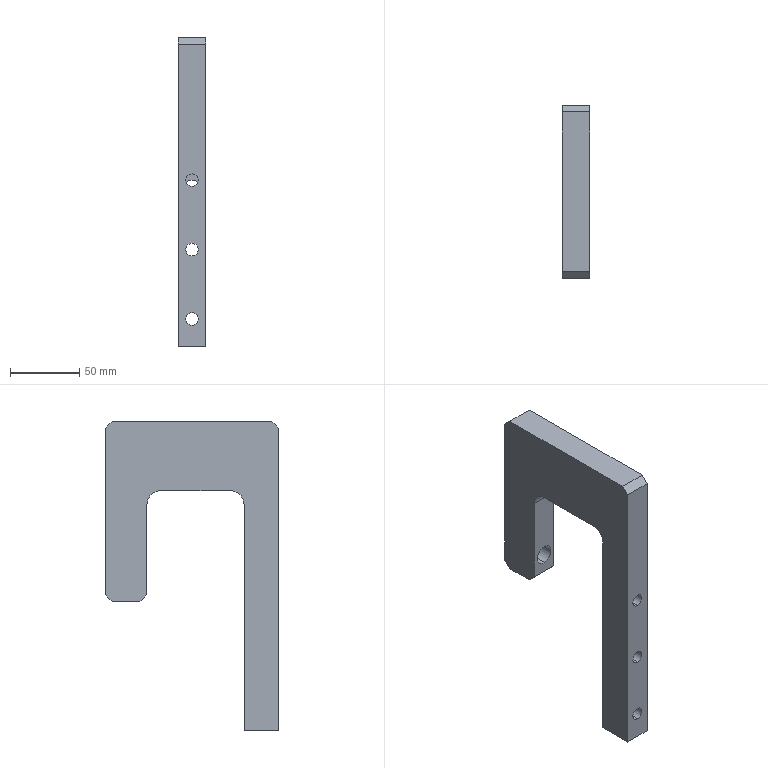Part | SolidWorks | features Chamfer 2, HoleWzd 2, ICE 2, Extrusion 1, Fillet 1, LPattern 1 | 1 solid | 33 faces | box 20 x 125 x 223 mm | volume 246915 mm3 | plane 17 | cylinder 16 | commonest cylinder face diameters 9 x6 15 x6 14 x2 20 x2
STEP:
#1=CARTESIAN_POINT('',(0.,82.5,120.));
#2=VERTEX_POINT('',#1);
#3=CARTESIAN_POINT('',(0.,82.5,106.));
#4=VERTEX_POINT('',#3);
#5=CARTESIAN_POINT('',(0.,82.5,113.));
#6=DIRECTION('',(0.,-1.,0.));
#7=DIRECTION('',(0.,0.,-1.));
#8=AXIS2_PLACEMENT_3D('',#5,#6,#7);
#9=CIRCLE('',#8,7.);
#10=EDGE_CURVE('',#2,#4,#9,.T.);
#11=ORIENTED_EDGE('',*,*,#10,.T.);
#12=CARTESIAN_POINT('',(0.,112.5,106.));
#13=VERTEX_POINT('',#12);
#14=CARTESIAN_POINT('',(0.,112.5,106.));
#15=DIRECTION('',(0.,1.,0.));
#16=VECTOR('',#15,1000.);
#17=LINE('',#14,#16);
#18=EDGE_CURVE('',#4,#13,#17,.T.);
#19=ORIENTED_EDGE('',*,*,#18,.T.);
#20=CARTESIAN_POINT('',(0.,112.5,120.));
#21=VERTEX_POINT('',#20);
#22=CARTESIAN_POINT('',(0.,112.5,113.));
#23=DIRECTION('',(0.,1.,0.));
#24=DIRECTION('',(0.,0.,1.));
#25=AXIS2_PLACEMENT_3D('',#22,#23,#24);
#26=CIRCLE('',#25,7.);
#27=EDGE_CURVE('',#13,#21,#26,.T.);
#28=ORIENTED_EDGE('',*,*,#27,.T.);
#29=CARTESIAN_POINT('',(0.,112.5,120.));
#30=DIRECTION('',(0.,1.,0.));
#31=VECTOR('',#30,1000.);
#32=LINE('',#29,#31);
#33=EDGE_CURVE('',#2,#21,#32,.T.);
#34=ORIENTED_EDGE('',*,*,#33,.F.);
#35=EDGE_LOOP('',(#11,#19,#28,#34));
#36=FACE_OUTER_BOUND('',#35,.T.);
#37=CARTESIAN_POINT('',(0.,112.5,113.));
#38=DIRECTION('',(0.,1.,0.));
#39=DIRECTION('',(0.,0.,1.));
#40=AXIS2_PLACEMENT_3D('',#37,#38,#39);
#41=CYLINDRICAL_SURFACE('',#40,7.);
#42=ADVANCED_FACE('',(#36),#41,.F.);
#43=CARTESIAN_POINT('',(0.,3.5,62.5));
#44=VERTEX_POINT('',#43);
#45=CARTESIAN_POINT('',(0.,3.5,77.5));
#46=VERTEX_POINT('',#45);
#47=CARTESIAN_POINT('',(0.,3.5,70.));
#48=DIRECTION('',(0.,1.,0.));
#49=DIRECTION('',(0.,0.,1.));
#50=AXIS2_PLACEMENT_3D('',#47,#48,#49);
#51=CIRCLE('',#50,7.5);
#52=EDGE_CURVE('',#44,#46,#51,.T.);
#53=ORIENTED_EDGE('',*,*,#52,.F.);
#54=CARTESIAN_POINT('',(0.,12.5,62.5));
#55=VERTEX_POINT('',#54);
#56=CARTESIAN_POINT('',(0.,12.5,62.5));
#57=DIRECTION('',(0.,1.,0.));
#58=VECTOR('',#57,1000.);
#59=LINE('',#56,#58);
#60=EDGE_CURVE('',#44,#55,#59,.T.);
#61=ORIENTED_EDGE('',*,*,#60,.T.);
#62=CARTESIAN_POINT('',(0.,12.5,77.5));
#63=VERTEX_POINT('',#62);
#64=CARTESIAN_POINT('',(0.,12.5,70.));
#65=DIRECTION('',(0.,1.,0.));
#66=DIRECTION('',(0.,0.,1.));
#67=AXIS2_PLACEMENT_3D('',#64,#65,#66);
#68=CIRCLE('',#67,7.5);
#69=EDGE_CURVE('',#55,#63,#68,.T.);
#70=ORIENTED_EDGE('',*,*,#69,.T.);
#71=CARTESIAN_POINT('',(0.,12.5,77.5));
#72=DIRECTION('',(0.,1.,0.));
#73=VECTOR('',#72,1000.);
#74=LINE('',#71,#73);
#75=EDGE_CURVE('',#46,#63,#74,.T.);
#76=ORIENTED_EDGE('',*,*,#75,.F.);
#77=EDGE_LOOP('',(#53,#61,#70,#76));
#78=FACE_OUTER_BOUND('',#77,.T.);
#79=CARTESIAN_POINT('',(0.,12.5,70.));
#80=DIRECTION('',(0.,1.,0.));
#81=DIRECTION('',(0.,0.,1.));
#82=AXIS2_PLACEMENT_3D('',#79,#80,#81);
#83=CYLINDRICAL_SURFACE('',#82,7.5);
#84=ADVANCED_FACE('',(#78),#83,.F.);
#85=CARTESIAN_POINT('',(0.,-12.5,65.5));
#86=VERTEX_POINT('',#85);
#87=CARTESIAN_POINT('',(0.,-12.5,74.5));
#88=VERTEX_POINT('',#87);
#89=CARTESIAN_POINT('',(0.,-12.5,70.));
#90=DIRECTION('',(0.,1.,0.));
#91=DIRECTION('',(0.,0.,1.));
#92=AXIS2_PLACEMENT_3D('',#89,#90,#91);
#93=CIRCLE('',#92,4.5);
#94=EDGE_CURVE('',#86,#88,#93,.T.);
#95=ORIENTED_EDGE('',*,*,#94,.F.);
#96=CARTESIAN_POINT('',(0.,3.5,65.5));
#97=VERTEX_POINT('',#96);
#98=CARTESIAN_POINT('',(0.,12.5,65.5));
#99=DIRECTION('',(0.,1.,0.));
#100=VECTOR('',#99,1000.);
#101=LINE('',#98,#100);
#102=EDGE_CURVE('',#86,#97,#101,.T.);
#103=ORIENTED_EDGE('',*,*,#102,.T.);
#104=CARTESIAN_POINT('',(0.,3.5,74.5));
#105=VERTEX_POINT('',#104);
#106=CARTESIAN_POINT('',(0.,3.5,70.));
#107=DIRECTION('',(0.,1.,0.));
#108=DIRECTION('',(0.,0.,1.));
#109=AXIS2_PLACEMENT_3D('',#106,#107,#108);
#110=CIRCLE('',#109,4.5);
#111=EDGE_CURVE('',#97,#105,#110,.T.);
#112=ORIENTED_EDGE('',*,*,#111,.T.);
#113=CARTESIAN_POINT('',(0.,12.5,74.5));
#114=DIRECTION('',(0.,1.,0.));
#115=VECTOR('',#114,1000.);
#116=LINE('',#113,#115);
#117=EDGE_CURVE('',#88,#105,#116,.T.);
#118=ORIENTED_EDGE('',*,*,#117,.F.);
#119=EDGE_LOOP('',(#95,#103,#112,#118));
#120=FACE_OUTER_BOUND('',#119,.T.);
#121=CARTESIAN_POINT('',(0.,12.5,70.));
#122=DIRECTION('',(0.,1.,0.));
#123=DIRECTION('',(0.,0.,1.));
#124=AXIS2_PLACEMENT_3D('',#121,#122,#123);
#125=CYLINDRICAL_SURFACE('',#124,4.5);
#126=ADVANCED_FACE('',(#120),#125,.F.);
#127=CARTESIAN_POINT('',(0.,3.5,12.5));
#128=VERTEX_POINT('',#127);
#129=CARTESIAN_POINT('',(0.,3.5,27.5));
#130=VERTEX_POINT('',#129);
#131=CARTESIAN_POINT('',(0.,3.5,20.));
#132=DIRECTION('',(0.,1.,0.));
#133=DIRECTION('',(0.,0.,1.));
#134=AXIS2_PLACEMENT_3D('',#131,#132,#133);
#135=CIRCLE('',#134,7.5);
#136=EDGE_CURVE('',#128,#130,#135,.T.);
#137=ORIENTED_EDGE('',*,*,#136,.F.);
#138=CARTESIAN_POINT('',(0.,12.5,12.5));
#139=VERTEX_POINT('',#138);
#140=CARTESIAN_POINT('',(0.,12.5,12.5));
#141=DIRECTION('',(0.,1.,0.));
#142=VECTOR('',#141,1000.);
#143=LINE('',#140,#142);
#144=EDGE_CURVE('',#128,#139,#143,.T.);
#145=ORIENTED_EDGE('',*,*,#144,.T.);
#146=CARTESIAN_POINT('',(0.,12.5,27.5));
#147=VERTEX_POINT('',#146);
#148=CARTESIAN_POINT('',(0.,12.5,20.));
#149=DIRECTION('',(0.,1.,0.));
#150=DIRECTION('',(0.,0.,1.));
#151=AXIS2_PLACEMENT_3D('',#148,#149,#150);
#152=CIRCLE('',#151,7.5);
#153=EDGE_CURVE('',#139,#147,#152,.T.);
#154=ORIENTED_EDGE('',*,*,#153,.T.);
#155=CARTESIAN_POINT('',(0.,12.5,27.5));
#156=DIRECTION('',(0.,1.,0.));
#157=VECTOR('',#156,1000.);
#158=LINE('',#155,#157);
#159=EDGE_CURVE('',#130,#147,#158,.T.);
#160=ORIENTED_EDGE('',*,*,#159,.F.);
#161=EDGE_LOOP('',(#137,#145,#154,#160));
#162=FACE_OUTER_BOUND('',#161,.T.);
#163=CARTESIAN_POINT('',(0.,12.5,20.));
#164=DIRECTION('',(0.,1.,0.));
#165=DIRECTION('',(0.,0.,1.));
#166=AXIS2_PLACEMENT_3D('',#163,#164,#165);
#167=CYLINDRICAL_SURFACE('',#166,7.5);
#168=ADVANCED_FACE('',(#162),#167,.F.);
#169=CARTESIAN_POINT('',(0.,-12.5,15.5));
#170=VERTEX_POINT('',#169);
#171=CARTESIAN_POINT('',(0.,-12.5,24.5));
#172=VERTEX_POINT('',#171);
#173=CARTESIAN_POINT('',(0.,-12.5,20.));
#174=DIRECTION('',(0.,1.,0.));
#175=DIRECTION('',(0.,0.,1.));
#176=AXIS2_PLACEMENT_3D('',#173,#174,#175);
#177=CIRCLE('',#176,4.5);
#178=EDGE_CURVE('',#170,#172,#177,.T.);
#179=ORIENTED_EDGE('',*,*,#178,.F.);
#180=CARTESIAN_POINT('',(0.,3.5,15.5));
#181=VERTEX_POINT('',#180);
#182=CARTESIAN_POINT('',(0.,12.5,15.5));
#183=DIRECTION('',(0.,1.,0.));
#184=VECTOR('',#183,1000.);
#185=LINE('',#182,#184);
#186=EDGE_CURVE('',#170,#181,#185,.T.);
#187=ORIENTED_EDGE('',*,*,#186,.T.);
#188=CARTESIAN_POINT('',(0.,3.5,24.5));
#189=VERTEX_POINT('',#188);
#190=CARTESIAN_POINT('',(0.,3.5,20.));
#191=DIRECTION('',(0.,1.,0.));
#192=DIRECTION('',(0.,0.,1.));
#193=AXIS2_PLACEMENT_3D('',#190,#191,#192);
#194=CIRCLE('',#193,4.5);
#195=EDGE_CURVE('',#181,#189,#194,.T.);
#196=ORIENTED_EDGE('',*,*,#195,.T.);
#197=CARTESIAN_POINT('',(0.,12.5,24.5));
#198=DIRECTION('',(0.,1.,0.));
#199=VECTOR('',#198,1000.);
#200=LINE('',#197,#199);
#201=EDGE_CURVE('',#172,#189,#200,.T.);
#202=ORIENTED_EDGE('',*,*,#201,.F.);
#203=EDGE_LOOP('',(#179,#187,#196,#202));
#204=FACE_OUTER_BOUND('',#203,.T.);
#205=CARTESIAN_POINT('',(0.,12.5,20.));
#206=DIRECTION('',(0.,1.,0.));
#207=DIRECTION('',(0.,0.,1.));
#208=AXIS2_PLACEMENT_3D('',#205,#206,#207);
#209=CYLINDRICAL_SURFACE('',#208,4.5);
#210=ADVANCED_FACE('',(#204),#209,.F.);
#211=CARTESIAN_POINT('',(0.,-12.5,115.5));
#212=VERTEX_POINT('',#211);
#213=CARTESIAN_POINT('',(0.,-12.5,124.5));
#214=VERTEX_POINT('',#213);
#215=CARTESIAN_POINT('',(0.,-12.5,120.));
#216=DIRECTION('',(0.,1.,0.));
#217=DIRECTION('',(0.,0.,1.));
#218=AXIS2_PLACEMENT_3D('',#215,#216,#217);
#219=CIRCLE('',#218,4.5);
#220=EDGE_CURVE('',#212,#214,#219,.T.);
#221=ORIENTED_EDGE('',*,*,#220,.F.);
#222=CARTESIAN_POINT('',(0.,3.5,115.5));
#223=VERTEX_POINT('',#222);
#224=CARTESIAN_POINT('',(0.,12.5,115.5));
#225=DIRECTION('',(0.,1.,0.));
#226=VECTOR('',#225,1000.);
#227=LINE('',#224,#226);
#228=EDGE_CURVE('',#212,#223,#227,.T.);
#229=ORIENTED_EDGE('',*,*,#228,.T.);
#230=CARTESIAN_POINT('',(0.,3.5,124.5));
#231=VERTEX_POINT('',#230);
#232=CARTESIAN_POINT('',(0.,3.5,120.));
#233=DIRECTION('',(0.,1.,0.));
#234=DIRECTION('',(0.,0.,1.));
#235=AXIS2_PLACEMENT_3D('',#232,#233,#234);
#236=CIRCLE('',#235,4.5);
#237=EDGE_CURVE('',#223,#231,#236,.T.);
#238=ORIENTED_EDGE('',*,*,#237,.T.);
#239=CARTESIAN_POINT('',(0.,12.5,124.5));
#240=DIRECTION('',(0.,1.,0.));
#241=VECTOR('',#240,1000.);
#242=LINE('',#239,#241);
#243=EDGE_CURVE('',#214,#231,#242,.T.);
#244=ORIENTED_EDGE('',*,*,#243,.F.);
#245=EDGE_LOOP('',(#221,#229,#238,#244));
#246=FACE_OUTER_BOUND('',#245,.T.);
#247=CARTESIAN_POINT('',(0.,12.5,120.));
#248=DIRECTION('',(0.,1.,0.));
#249=DIRECTION('',(0.,0.,1.));
#250=AXIS2_PLACEMENT_3D('',#247,#248,#249);
#251=CYLINDRICAL_SURFACE('',#250,4.5);
#252=ADVANCED_FACE('',(#246),#251,.F.);
#253=CARTESIAN_POINT('',(0.,3.5,112.5));
#254=VERTEX_POINT('',#253);
#255=CARTESIAN_POINT('',(0.,3.5,127.5));
#256=VERTEX_POINT('',#255);
#257=CARTESIAN_POINT('',(0.,3.5,120.));
#258=DIRECTION('',(0.,1.,0.));
#259=DIRECTION('',(0.,0.,1.));
#260=AXIS2_PLACEMENT_3D('',#257,#258,#259);
#261=CIRCLE('',#260,7.5);
#262=EDGE_CURVE('',#254,#256,#261,.T.);
#263=ORIENTED_EDGE('',*,*,#262,.F.);
#264=CARTESIAN_POINT('',(0.,12.5,112.5));
#265=VERTEX_POINT('',#264);
#266=CARTESIAN_POINT('',(0.,12.5,112.5));
#267=DIRECTION('',(0.,1.,0.));
#268=VECTOR('',#267,1000.);
#269=LINE('',#266,#268);
#270=EDGE_CURVE('',#254,#265,#269,.T.);
#271=ORIENTED_EDGE('',*,*,#270,.T.);
#272=CARTESIAN_POINT('',(0.,12.5,127.5));
#273=VERTEX_POINT('',#272);
#274=CARTESIAN_POINT('',(0.,12.5,120.));
#275=DIRECTION('',(0.,1.,0.));
#276=DIRECTION('',(0.,0.,1.));
#277=AXIS2_PLACEMENT_3D('',#274,#275,#276);
#278=CIRCLE('',#277,7.5);
#279=EDGE_CURVE('',#265,#273,#278,.T.);
#280=ORIENTED_EDGE('',*,*,#279,.T.);
#281=CARTESIAN_POINT('',(0.,12.5,127.5));
#282=DIRECTION('',(0.,1.,0.));
#283=VECTOR('',#282,1000.);
#284=LINE('',#281,#283);
#285=EDGE_CURVE('',#256,#273,#284,.T.);
#286=ORIENTED_EDGE('',*,*,#285,.F.);
#287=EDGE_LOOP('',(#263,#271,#280,#286));
#288=FACE_OUTER_BOUND('',#287,.T.);
#289=CARTESIAN_POINT('',(0.,12.5,120.));
#290=DIRECTION('',(0.,1.,0.));
#291=DIRECTION('',(0.,0.,1.));
#292=AXIS2_PLACEMENT_3D('',#289,#290,#291);
#293=CYLINDRICAL_SURFACE('',#292,7.5);
#294=ADVANCED_FACE('',(#288),#293,.F.);
#295=CARTESIAN_POINT('',(0.,12.5,120.));
#296=DIRECTION('',(0.,1.,0.));
#297=DIRECTION('',(0.,0.,1.));
#298=AXIS2_PLACEMENT_3D('',#295,#296,#297);
#299=CIRCLE('',#298,7.5);
#300=EDGE_CURVE('',#273,#265,#299,.T.);
#301=ORIENTED_EDGE('',*,*,#300,.F.);
#302=ORIENTED_EDGE('',*,*,#279,.F.);
#303=EDGE_LOOP('',(#301,#302));
#304=FACE_BOUND('',#303,.T.);
#305=CARTESIAN_POINT('',(0.,12.5,20.));
#306=DIRECTION('',(0.,1.,0.));
#307=DIRECTION('',(0.,0.,1.));
#308=AXIS2_PLACEMENT_3D('',#305,#306,#307);
#309=CIRCLE('',#308,7.5);
#310=EDGE_CURVE('',#147,#139,#309,.T.);
#311=ORIENTED_EDGE('',*,*,#310,.F.);
#312=ORIENTED_EDGE('',*,*,#153,.F.);
#313=EDGE_LOOP('',(#311,#312));
#314=FACE_BOUND('',#313,.T.);
#315=CARTESIAN_POINT('',(0.,12.5,70.));
#316=DIRECTION('',(0.,1.,0.));
#317=DIRECTION('',(0.,0.,1.));
#318=AXIS2_PLACEMENT_3D('',#315,#316,#317);
#319=CIRCLE('',#318,7.5);
#320=EDGE_CURVE('',#63,#55,#319,.T.);
#321=ORIENTED_EDGE('',*,*,#320,.F.);
#322=ORIENTED_EDGE('',*,*,#69,.F.);
#323=EDGE_LOOP('',(#321,#322));
#324=FACE_BOUND('',#323,.T.);
#325=CARTESIAN_POINT('',(-10.,12.5,163.));
#326=VERTEX_POINT('',#325);
#327=CARTESIAN_POINT('',(-10.,12.5,0.));
#328=VERTEX_POINT('',#327);
#329=CARTESIAN_POINT('',(-10.,12.5,223.));
#330=DIRECTION('',(0.,0.,-1.));
#331=VECTOR('',#330,1000.);
#332=LINE('',#329,#331);
#333=EDGE_CURVE('',#326,#328,#332,.T.);
#334=ORIENTED_EDGE('',*,*,#333,.F.);
#335=CARTESIAN_POINT('',(10.,12.5,163.));
#336=VERTEX_POINT('',#335);
#337=CARTESIAN_POINT('',(10.,12.5,163.));
#338=DIRECTION('',(1.,0.,0.));
#339=VECTOR('',#338,1000.);
#340=LINE('',#337,#339);
#341=EDGE_CURVE('',#326,#336,#340,.T.);
#342=ORIENTED_EDGE('',*,*,#341,.T.);
#343=CARTESIAN_POINT('',(10.,12.5,0.));
#344=VERTEX_POINT('',#343);
#345=CARTESIAN_POINT('',(10.,12.5,223.));
#346=DIRECTION('',(0.,0.,-1.));
#347=VECTOR('',#346,1000.);
#348=LINE('',#345,#347);
#349=EDGE_CURVE('',#336,#344,#348,.T.);
#350=ORIENTED_EDGE('',*,*,#349,.T.);
#351=CARTESIAN_POINT('',(-10.,12.5,0.));
#352=DIRECTION('',(-1.,0.,0.));
#353=VECTOR('',#352,1000.);
#354=LINE('',#351,#353);
#355=EDGE_CURVE('',#344,#328,#354,.T.);
#356=ORIENTED_EDGE('',*,*,#355,.T.);
#357=EDGE_LOOP('',(#334,#342,#350,#356));
#358=FACE_OUTER_BOUND('',#357,.T.);
#359=CARTESIAN_POINT('',(-10.,12.5,223.));
#360=DIRECTION('',(0.,-1.,0.));
#361=DIRECTION('',(0.,0.,-1.));
#362=AXIS2_PLACEMENT_3D('',#359,#360,#361);
#363=PLANE('',#362);
#364=ADVANCED_FACE('',(#304,#314,#324,#358),#363,.F.);
#365=ORIENTED_EDGE('',*,*,#270,.F.);
#366=CARTESIAN_POINT('',(0.,3.5,120.));
#367=DIRECTION('',(0.,1.,0.));
#368=DIRECTION('',(0.,0.,1.));
#369=AXIS2_PLACEMENT_3D('',#366,#367,#368);
#370=CIRCLE('',#369,7.5);
#371=EDGE_CURVE('',#256,#254,#370,.T.);
#372=ORIENTED_EDGE('',*,*,#371,.F.);
#373=ORIENTED_EDGE('',*,*,#285,.T.);
#374=ORIENTED_EDGE('',*,*,#300,.T.);
#375=EDGE_LOOP('',(#365,#372,#373,#374));
#376=FACE_OUTER_BOUND('',#375,.T.);
#377=CARTESIAN_POINT('',(0.,12.5,120.));
#378=DIRECTION('',(0.,1.,0.));
#379=DIRECTION('',(0.,0.,1.));
#380=AXIS2_PLACEMENT_3D('',#377,#378,#379);
#381=CYLINDRICAL_SURFACE('',#380,7.5);
#382=ADVANCED_FACE('',(#376),#381,.F.);
#383=CARTESIAN_POINT('',(0.,3.5,120.));
#384=DIRECTION('',(0.,1.,0.));
#385=DIRECTION('',(0.,0.,1.));
#386=AXIS2_PLACEMENT_3D('',#383,#384,#385);
#387=CIRCLE('',#386,4.5);
#388=EDGE_CURVE('',#231,#223,#387,.T.);
#389=ORIENTED_EDGE('',*,*,#388,.F.);
#390=ORIENTED_EDGE('',*,*,#237,.F.);
#391=EDGE_LOOP('',(#389,#390));
#392=FACE_BOUND('',#391,.T.);
#393=ORIENTED_EDGE('',*,*,#371,.T.);
#394=ORIENTED_EDGE('',*,*,#262,.T.);
#395=EDGE_LOOP('',(#393,#394));
#396=FACE_OUTER_BOUND('',#395,.T.);
#397=CARTESIAN_POINT('',(4.5,3.5,120.));
#398=DIRECTION('',(0.,-1.,0.));
#399=DIRECTION('',(0.,0.,-1.));
#400=AXIS2_PLACEMENT_3D('',#397,#398,#399);
#401=PLANE('',#400);
#402=ADVANCED_FACE('',(#392,#396),#401,.F.);
#403=ORIENTED_EDGE('',*,*,#228,.F.);
#404=CARTESIAN_POINT('',(0.,-12.5,120.));
#405=DIRECTION('',(0.,1.,0.));
#406=DIRECTION('',(0.,0.,1.));
#407=AXIS2_PLACEMENT_3D('',#404,#405,#406);
#408=CIRCLE('',#407,4.5);
#409=EDGE_CURVE('',#214,#212,#408,.T.);
#410=ORIENTED_EDGE('',*,*,#409,.F.);
#411=ORIENTED_EDGE('',*,*,#243,.T.);
#412=ORIENTED_EDGE('',*,*,#388,.T.);
#413=EDGE_LOOP('',(#403,#410,#411,#412));
#414=FACE_OUTER_BOUND('',#413,.T.);
#415=CARTESIAN_POINT('',(0.,12.5,120.));
#416=DIRECTION('',(0.,1.,0.));
#417=DIRECTION('',(0.,0.,1.));
#418=AXIS2_PLACEMENT_3D('',#415,#416,#417);
#419=CYLINDRICAL_SURFACE('',#418,4.5);
#420=ADVANCED_FACE('',(#414),#419,.F.);
#421=CARTESIAN_POINT('',(10.,-7.5,223.));
#422=VERTEX_POINT('',#421);
#423=CARTESIAN_POINT('',(10.,107.5,223.));
#424=VERTEX_POINT('',#423);
#425=CARTESIAN_POINT('',(10.,12.5,223.));
#426=DIRECTION('',(0.,1.,0.));
#427=VECTOR('',#426,1000.);
#428=LINE('',#425,#427);
#429=EDGE_CURVE('',#422,#424,#428,.T.);
#430=ORIENTED_EDGE('',*,*,#429,.F.);
#431=CARTESIAN_POINT('',(10.,-12.5,218.));
#432=VERTEX_POINT('',#431);
#433=CARTESIAN_POINT('',(10.,-7.5,223.));
#434=DIRECTION('',(0.,-0.7071,-0.7071));
#435=VECTOR('',#434,1000.);
#436=LINE('',#433,#435);
#437=EDGE_CURVE('',#422,#432,#436,.T.);
#438=ORIENTED_EDGE('',*,*,#437,.T.);
#439=CARTESIAN_POINT('',(10.,-12.5,0.));
#440=VERTEX_POINT('',#439);
#441=CARTESIAN_POINT('',(10.,-12.5,223.));
#442=DIRECTION('',(0.,0.,-1.));
#443=VECTOR('',#442,1000.);
#444=LINE('',#441,#443);
#445=EDGE_CURVE('',#432,#440,#444,.T.);
#446=ORIENTED_EDGE('',*,*,#445,.T.);
#447=CARTESIAN_POINT('',(10.,12.5,0.));
#448=DIRECTION('',(0.,1.,0.));
#449=VECTOR('',#448,1000.);
#450=LINE('',#447,#449);
#451=EDGE_CURVE('',#440,#344,#450,.T.);
#452=ORIENTED_EDGE('',*,*,#451,.T.);
#453=ORIENTED_EDGE('',*,*,#349,.F.);
#454=CARTESIAN_POINT('',(10.,22.5,173.));
#455=VERTEX_POINT('',#454);
#456=CARTESIAN_POINT('',(10.,22.5,163.));
#457=DIRECTION('',(-1.,0.,0.));
#458=DIRECTION('',(0.,-1.,0.));
#459=AXIS2_PLACEMENT_3D('',#456,#457,#458);
#460=CIRCLE('',#459,10.);
#461=EDGE_CURVE('',#336,#455,#460,.T.);
#462=ORIENTED_EDGE('',*,*,#461,.T.);
#463=CARTESIAN_POINT('',(10.,72.5,173.));
#464=VERTEX_POINT('',#463);
#465=CARTESIAN_POINT('',(10.,82.5,173.));
#466=DIRECTION('',(0.,-1.,0.));
#467=VECTOR('',#466,1000.);
#468=LINE('',#465,#467);
#469=EDGE_CURVE('',#464,#455,#468,.T.);
#470=ORIENTED_EDGE('',*,*,#469,.F.);
#471=CARTESIAN_POINT('',(10.,82.5,163.));
#472=VERTEX_POINT('',#471);
#473=CARTESIAN_POINT('',(10.,72.5,163.));
#474=DIRECTION('',(-1.,0.,0.));
#475=DIRECTION('',(0.,-1.,0.));
#476=AXIS2_PLACEMENT_3D('',#473,#474,#475);
#477=CIRCLE('',#476,10.);
#478=EDGE_CURVE('',#464,#472,#477,.T.);
#479=ORIENTED_EDGE('',*,*,#478,.T.);
#480=CARTESIAN_POINT('',(10.,82.5,98.));
#481=VERTEX_POINT('',#480);
#482=CARTESIAN_POINT('',(10.,82.5,223.));
#483=DIRECTION('',(0.,0.,-1.));
#484=VECTOR('',#483,1000.);
#485=LINE('',#482,#484);
#486=EDGE_CURVE('',#472,#481,#485,.T.);
#487=ORIENTED_EDGE('',*,*,#486,.T.);
#488=CARTESIAN_POINT('',(10.,87.5,93.));
#489=VERTEX_POINT('',#488);
#490=CARTESIAN_POINT('',(10.,87.5,93.));
#491=DIRECTION('',(0.,0.7071,-0.7071));
#492=VECTOR('',#491,1000.);
#493=LINE('',#490,#492);
#494=EDGE_CURVE('',#481,#489,#493,.T.);
#495=ORIENTED_EDGE('',*,*,#494,.T.);
#496=CARTESIAN_POINT('',(10.,107.5,93.));
#497=VERTEX_POINT('',#496);
#498=CARTESIAN_POINT('',(10.,112.5,93.));
#499=DIRECTION('',(0.,-1.,0.));
#500=VECTOR('',#499,1000.);
#501=LINE('',#498,#500);
#502=EDGE_CURVE('',#497,#489,#501,.T.);
#503=ORIENTED_EDGE('',*,*,#502,.F.);
#504=CARTESIAN_POINT('',(10.,112.5,98.));
#505=VERTEX_POINT('',#504);
#506=CARTESIAN_POINT('',(10.,112.5,98.));
#507=DIRECTION('',(0.,0.7071,0.7071));
#508=VECTOR('',#507,1000.);
#509=LINE('',#506,#508);
#510=EDGE_CURVE('',#497,#505,#509,.T.);
#511=ORIENTED_EDGE('',*,*,#510,.T.);
#512=CARTESIAN_POINT('',(10.,112.5,218.));
#513=VERTEX_POINT('',#512);
#514=CARTESIAN_POINT('',(10.,112.5,223.));
#515=DIRECTION('',(0.,0.,-1.));
#516=VECTOR('',#515,1000.);
#517=LINE('',#514,#516);
#518=EDGE_CURVE('',#513,#505,#517,.T.);
#519=ORIENTED_EDGE('',*,*,#518,.F.);
#520=CARTESIAN_POINT('',(10.,112.5,218.));
#521=DIRECTION('',(0.,-0.7071,0.7071));
#522=VECTOR('',#521,1000.);
#523=LINE('',#520,#522);
#524=EDGE_CURVE('',#513,#424,#523,.T.);
#525=ORIENTED_EDGE('',*,*,#524,.T.);
#526=EDGE_LOOP('',(#430,#438,#446,#452,#453,#462,#470,#479,#487,#495,#503,#511,#519,#525));
#527=FACE_OUTER_BOUND('',#526,.T.);
#528=CARTESIAN_POINT('',(10.,12.5,223.));
#529=DIRECTION('',(-1.,0.,0.));
#530=DIRECTION('',(0.,-1.,0.));
#531=AXIS2_PLACEMENT_3D('',#528,#529,#530);
#532=PLANE('',#531);
#533=ADVANCED_FACE('',(#527),#532,.F.);
#534=CARTESIAN_POINT('',(-10.,-12.5,218.));
#535=VERTEX_POINT('',#534);
#536=CARTESIAN_POINT('',(-10.,-12.5,0.));
#537=VERTEX_POINT('',#536);
#538=CARTESIAN_POINT('',(-10.,-12.5,223.));
#539=DIRECTION('',(0.,0.,-1.));
#540=VECTOR('',#539,1000.);
#541=LINE('',#538,#540);
#542=EDGE_CURVE('',#535,#537,#541,.T.);
#543=ORIENTED_EDGE('',*,*,#542,.F.);
#544=CARTESIAN_POINT('',(-10.,-7.5,223.));
#545=VERTEX_POINT('',#544);
#546=CARTESIAN_POINT('',(-10.,-7.5,223.));
#547=DIRECTION('',(0.,0.7071,0.7071));
#548=VECTOR('',#547,1000.);
#549=LINE('',#546,#548);
#550=EDGE_CURVE('',#535,#545,#549,.T.);
#551=ORIENTED_EDGE('',*,*,#550,.T.);
#552=CARTESIAN_POINT('',(-10.,107.5,223.));
#553=VERTEX_POINT('',#552);
#554=CARTESIAN_POINT('',(-10.,12.5,223.));
#555=DIRECTION('',(0.,-1.,0.));
#556=VECTOR('',#555,1000.);
#557=LINE('',#554,#556);
#558=EDGE_CURVE('',#553,#545,#557,.T.);
#559=ORIENTED_EDGE('',*,*,#558,.F.);
#560=CARTESIAN_POINT('',(-10.,112.5,218.));
#561=VERTEX_POINT('',#560);
#562=CARTESIAN_POINT('',(-10.,112.5,218.));
#563=DIRECTION('',(0.,0.7071,-0.7071));
#564=VECTOR('',#563,1000.);
#565=LINE('',#562,#564);
#566=EDGE_CURVE('',#553,#561,#565,.T.);
#567=ORIENTED_EDGE('',*,*,#566,.T.);
#568=CARTESIAN_POINT('',(-10.,112.5,98.));
#569=VERTEX_POINT('',#568);
#570=CARTESIAN_POINT('',(-10.,112.5,223.));
#571=DIRECTION('',(0.,0.,1.));
#572=VECTOR('',#571,1000.);
#573=LINE('',#570,#572);
#574=EDGE_CURVE('',#569,#561,#573,.T.);
#575=ORIENTED_EDGE('',*,*,#574,.F.);
#576=CARTESIAN_POINT('',(-10.,107.5,93.));
#577=VERTEX_POINT('',#576);
#578=CARTESIAN_POINT('',(-10.,112.5,98.));
#579=DIRECTION('',(0.,-0.7071,-0.7071));
#580=VECTOR('',#579,1000.);
#581=LINE('',#578,#580);
#582=EDGE_CURVE('',#569,#577,#581,.T.);
#583=ORIENTED_EDGE('',*,*,#582,.T.);
#584=CARTESIAN_POINT('',(-10.,87.5,93.));
#585=VERTEX_POINT('',#584);
#586=CARTESIAN_POINT('',(-10.,112.5,93.));
#587=DIRECTION('',(0.,-1.,0.));
#588=VECTOR('',#587,1000.);
#589=LINE('',#586,#588);
#590=EDGE_CURVE('',#577,#585,#589,.T.);
#591=ORIENTED_EDGE('',*,*,#590,.T.);
#592=CARTESIAN_POINT('',(-10.,82.5,98.));
#593=VERTEX_POINT('',#592);
#594=CARTESIAN_POINT('',(-10.,87.5,93.));
#595=DIRECTION('',(0.,-0.7071,0.7071));
#596=VECTOR('',#595,1000.);
#597=LINE('',#594,#596);
#598=EDGE_CURVE('',#585,#593,#597,.T.);
#599=ORIENTED_EDGE('',*,*,#598,.T.);
#600=CARTESIAN_POINT('',(-10.,82.5,163.));
#601=VERTEX_POINT('',#600);
#602=CARTESIAN_POINT('',(-10.,82.5,223.));
#603=DIRECTION('',(0.,0.,1.));
#604=VECTOR('',#603,1000.);
#605=LINE('',#602,#604);
#606=EDGE_CURVE('',#593,#601,#605,.T.);
#607=ORIENTED_EDGE('',*,*,#606,.T.);
#608=CARTESIAN_POINT('',(-10.,72.5,173.));
#609=VERTEX_POINT('',#608);
#610=CARTESIAN_POINT('',(-10.,72.5,163.));
#611=DIRECTION('',(1.,0.,0.));
#612=DIRECTION('',(0.,1.,0.));
#613=AXIS2_PLACEMENT_3D('',#610,#611,#612);
#614=CIRCLE('',#613,10.);
#615=EDGE_CURVE('',#601,#609,#614,.T.);
#616=ORIENTED_EDGE('',*,*,#615,.T.);
#617=CARTESIAN_POINT('',(-10.,22.5,173.));
#618=VERTEX_POINT('',#617);
#619=CARTESIAN_POINT('',(-10.,82.5,173.));
#620=DIRECTION('',(0.,-1.,0.));
#621=VECTOR('',#620,1000.);
#622=LINE('',#619,#621);
#623=EDGE_CURVE('',#609,#618,#622,.T.);
#624=ORIENTED_EDGE('',*,*,#623,.T.);
#625=CARTESIAN_POINT('',(-10.,22.5,163.));
#626=DIRECTION('',(1.,0.,0.));
#627=DIRECTION('',(0.,1.,0.));
#628=AXIS2_PLACEMENT_3D('',#625,#626,#627);
#629=CIRCLE('',#628,10.);
#630=EDGE_CURVE('',#618,#326,#629,.T.);
#631=ORIENTED_EDGE('',*,*,#630,.T.);
#632=ORIENTED_EDGE('',*,*,#333,.T.);
#633=CARTESIAN_POINT('',(-10.,12.5,0.));
#634=DIRECTION('',(0.,-1.,0.));
#635=VECTOR('',#634,1000.);
#636=LINE('',#633,#635);
#637=EDGE_CURVE('',#328,#537,#636,.T.);
#638=ORIENTED_EDGE('',*,*,#637,.T.);
#639=EDGE_LOOP('',(#543,#551,#559,#567,#575,#583,#591,#599,#607,#616,#624,#631,#632,#638));
#640=FACE_OUTER_BOUND('',#639,.T.);
#641=CARTESIAN_POINT('',(-10.,12.5,223.));
#642=DIRECTION('',(1.,0.,0.));
#643=DIRECTION('',(0.,1.,0.));
#644=AXIS2_PLACEMENT_3D('',#641,#642,#643);
#645=PLANE('',#644);
#646=ADVANCED_FACE('',(#640),#645,.F.);
#647=CARTESIAN_POINT('',(0.,-12.5,70.));
#648=DIRECTION('',(0.,1.,0.));
#649=DIRECTION('',(0.,0.,1.));
#650=AXIS2_PLACEMENT_3D('',#647,#648,#649);
#651=CIRCLE('',#650,4.5);
#652=EDGE_CURVE('',#88,#86,#651,.T.);
#653=ORIENTED_EDGE('',*,*,#652,.T.);
#654=ORIENTED_EDGE('',*,*,#94,.T.);
#655=EDGE_LOOP('',(#653,#654));
#656=FACE_BOUND('',#655,.T.);
#657=CARTESIAN_POINT('',(0.,-12.5,20.));
#658=DIRECTION('',(0.,1.,0.));
#659=DIRECTION('',(0.,0.,1.));
#660=AXIS2_PLACEMENT_3D('',#657,#658,#659);
#661=CIRCLE('',#660,4.5);
#662=EDGE_CURVE('',#172,#170,#661,.T.);
#663=ORIENTED_EDGE('',*,*,#662,.T.);
#664=ORIENTED_EDGE('',*,*,#178,.T.);
#665=EDGE_LOOP('',(#663,#664));
#666=FACE_BOUND('',#665,.T.);
#667=ORIENTED_EDGE('',*,*,#445,.F.);
#668=CARTESIAN_POINT('',(-10.,-12.5,218.));
#669=DIRECTION('',(-1.,0.,0.));
#670=VECTOR('',#669,1000.);
#671=LINE('',#668,#670);
#672=EDGE_CURVE('',#432,#535,#671,.T.);
#673=ORIENTED_EDGE('',*,*,#672,.T.);
#674=ORIENTED_EDGE('',*,*,#542,.T.);
#675=CARTESIAN_POINT('',(-10.,-12.5,0.));
#676=DIRECTION('',(1.,0.,0.));
#677=VECTOR('',#676,1000.);
#678=LINE('',#675,#677);
#679=EDGE_CURVE('',#537,#440,#678,.T.);
#680=ORIENTED_EDGE('',*,*,#679,.T.);
#681=EDGE_LOOP('',(#667,#673,#674,#680));
#682=FACE_OUTER_BOUND('',#681,.T.);
#683=ORIENTED_EDGE('',*,*,#409,.T.);
#684=ORIENTED_EDGE('',*,*,#220,.T.);
#685=EDGE_LOOP('',(#683,#684));
#686=FACE_BOUND('',#685,.T.);
#687=CARTESIAN_POINT('',(-10.,-12.5,223.));
#688=DIRECTION('',(0.,1.,0.));
#689=DIRECTION('',(0.,0.,1.));
#690=AXIS2_PLACEMENT_3D('',#687,#688,#689);
#691=PLANE('',#690);
#692=ADVANCED_FACE('',(#656,#666,#682,#686),#691,.F.);
#693=ORIENTED_EDGE('',*,*,#558,.T.);
#694=CARTESIAN_POINT('',(10.,-7.5,223.));
#695=DIRECTION('',(1.,0.,0.));
#696=VECTOR('',#695,1000.);
#697=LINE('',#694,#696);
#698=EDGE_CURVE('',#545,#422,#697,.T.);
#699=ORIENTED_EDGE('',*,*,#698,.T.);
#700=ORIENTED_EDGE('',*,*,#429,.T.);
#701=CARTESIAN_POINT('',(-10.,107.5,223.));
#702=DIRECTION('',(-1.,0.,0.));
#703=VECTOR('',#702,1000.);
#704=LINE('',#701,#703);
#705=EDGE_CURVE('',#424,#553,#704,.T.);
#706=ORIENTED_EDGE('',*,*,#705,.T.);
#707=EDGE_LOOP('',(#693,#699,#700,#706));
#708=FACE_OUTER_BOUND('',#707,.T.);
#709=CARTESIAN_POINT('',(0.,0.,223.));
#710=DIRECTION('',(0.,0.,1.));
#711=DIRECTION('',(1.,0.,0.));
#712=AXIS2_PLACEMENT_3D('',#709,#710,#711);
#713=PLANE('',#712);
#714=ADVANCED_FACE('',(#708),#713,.T.);
#715=ORIENTED_EDGE('',*,*,#451,.F.);
#716=ORIENTED_EDGE('',*,*,#679,.F.);
#717=ORIENTED_EDGE('',*,*,#637,.F.);
#718=ORIENTED_EDGE('',*,*,#355,.F.);
#719=EDGE_LOOP('',(#715,#716,#717,#718));
#720=FACE_OUTER_BOUND('',#719,.T.);
#721=CARTESIAN_POINT('',(0.,0.,0.));
#722=DIRECTION('',(0.,0.,1.));
#723=DIRECTION('',(1.,0.,0.));
#724=AXIS2_PLACEMENT_3D('',#721,#722,#723);
#725=PLANE('',#724);
#726=ADVANCED_FACE('',(#720),#725,.F.);
#727=ORIENTED_EDGE('',*,*,#186,.F.);
#728=ORIENTED_EDGE('',*,*,#662,.F.);
#729=ORIENTED_EDGE('',*,*,#201,.T.);
#730=CARTESIAN_POINT('',(0.,3.5,20.));
#731=DIRECTION('',(0.,1.,0.));
#732=DIRECTION('',(0.,0.,1.));
#733=AXIS2_PLACEMENT_3D('',#730,#731,#732);
#734=CIRCLE('',#733,4.5);
#735=EDGE_CURVE('',#189,#181,#734,.T.);
#736=ORIENTED_EDGE('',*,*,#735,.T.);
#737=EDGE_LOOP('',(#727,#728,#729,#736));
#738=FACE_OUTER_BOUND('',#737,.T.);
#739=CARTESIAN_POINT('',(0.,12.5,20.));
#740=DIRECTION('',(0.,1.,0.));
#741=DIRECTION('',(0.,0.,1.));
#742=AXIS2_PLACEMENT_3D('',#739,#740,#741);
#743=CYLINDRICAL_SURFACE('',#742,4.5);
#744=ADVANCED_FACE('',(#738),#743,.F.);
#745=ORIENTED_EDGE('',*,*,#735,.F.);
#746=ORIENTED_EDGE('',*,*,#195,.F.);
#747=EDGE_LOOP('',(#745,#746));
#748=FACE_BOUND('',#747,.T.);
#749=CARTESIAN_POINT('',(0.,3.5,20.));
#750=DIRECTION('',(0.,1.,0.));
#751=DIRECTION('',(0.,0.,1.));
#752=AXIS2_PLACEMENT_3D('',#749,#750,#751);
#753=CIRCLE('',#752,7.5);
#754=EDGE_CURVE('',#130,#128,#753,.T.);
#755=ORIENTED_EDGE('',*,*,#754,.T.);
#756=ORIENTED_EDGE('',*,*,#136,.T.);
#757=EDGE_LOOP('',(#755,#756));
#758=FACE_OUTER_BOUND('',#757,.T.);
#759=CARTESIAN_POINT('',(4.5,3.5,20.));
#760=DIRECTION('',(0.,-1.,0.));
#761=DIRECTION('',(0.,0.,-1.));
#762=AXIS2_PLACEMENT_3D('',#759,#760,#761);
#763=PLANE('',#762);
#764=ADVANCED_FACE('',(#748,#758),#763,.F.);
#765=ORIENTED_EDGE('',*,*,#144,.F.);
#766=ORIENTED_EDGE('',*,*,#754,.F.);
#767=ORIENTED_EDGE('',*,*,#159,.T.);
#768=ORIENTED_EDGE('',*,*,#310,.T.);
#769=EDGE_LOOP('',(#765,#766,#767,#768));
#770=FACE_OUTER_BOUND('',#769,.T.);
#771=CARTESIAN_POINT('',(0.,12.5,20.));
#772=DIRECTION('',(0.,1.,0.));
#773=DIRECTION('',(0.,0.,1.));
#774=AXIS2_PLACEMENT_3D('',#771,#772,#773);
#775=CYLINDRICAL_SURFACE('',#774,7.5);
#776=ADVANCED_FACE('',(#770),#775,.F.);
#777=ORIENTED_EDGE('',*,*,#102,.F.);
#778=ORIENTED_EDGE('',*,*,#652,.F.);
#779=ORIENTED_EDGE('',*,*,#117,.T.);
#780=CARTESIAN_POINT('',(0.,3.5,70.));
#781=DIRECTION('',(0.,1.,0.));
#782=DIRECTION('',(0.,0.,1.));
#783=AXIS2_PLACEMENT_3D('',#780,#781,#782);
#784=CIRCLE('',#783,4.5);
#785=EDGE_CURVE('',#105,#97,#784,.T.);
#786=ORIENTED_EDGE('',*,*,#785,.T.);
#787=EDGE_LOOP('',(#777,#778,#779,#786));
#788=FACE_OUTER_BOUND('',#787,.T.);
#789=CARTESIAN_POINT('',(0.,12.5,70.));
#790=DIRECTION('',(0.,1.,0.));
#791=DIRECTION('',(0.,0.,1.));
#792=AXIS2_PLACEMENT_3D('',#789,#790,#791);
#793=CYLINDRICAL_SURFACE('',#792,4.5);
#794=ADVANCED_FACE('',(#788),#793,.F.);
#795=ORIENTED_EDGE('',*,*,#785,.F.);
#796=ORIENTED_EDGE('',*,*,#111,.F.);
#797=EDGE_LOOP('',(#795,#796));
#798=FACE_BOUND('',#797,.T.);
#799=CARTESIAN_POINT('',(0.,3.5,70.));
#800=DIRECTION('',(0.,1.,0.));
#801=DIRECTION('',(0.,0.,1.));
#802=AXIS2_PLACEMENT_3D('',#799,#800,#801);
#803=CIRCLE('',#802,7.5);
#804=EDGE_CURVE('',#46,#44,#803,.T.);
#805=ORIENTED_EDGE('',*,*,#804,.T.);
#806=ORIENTED_EDGE('',*,*,#52,.T.);
#807=EDGE_LOOP('',(#805,#806));
#808=FACE_OUTER_BOUND('',#807,.T.);
#809=CARTESIAN_POINT('',(4.5,3.5,70.));
#810=DIRECTION('',(0.,-1.,0.));
#811=DIRECTION('',(0.,0.,-1.));
#812=AXIS2_PLACEMENT_3D('',#809,#810,#811);
#813=PLANE('',#812);
#814=ADVANCED_FACE('',(#798,#808),#813,.F.);
#815=ORIENTED_EDGE('',*,*,#60,.F.);
#816=ORIENTED_EDGE('',*,*,#804,.F.);
#817=ORIENTED_EDGE('',*,*,#75,.T.);
#818=ORIENTED_EDGE('',*,*,#320,.T.);
#819=EDGE_LOOP('',(#815,#816,#817,#818));
#820=FACE_OUTER_BOUND('',#819,.T.);
#821=CARTESIAN_POINT('',(0.,12.5,70.));
#822=DIRECTION('',(0.,1.,0.));
#823=DIRECTION('',(0.,0.,1.));
#824=AXIS2_PLACEMENT_3D('',#821,#822,#823);
#825=CYLINDRICAL_SURFACE('',#824,7.5);
#826=ADVANCED_FACE('',(#820),#825,.F.);
#827=ORIENTED_EDGE('',*,*,#623,.F.);
#828=CARTESIAN_POINT('',(-10.,72.5,173.));
#829=DIRECTION('',(1.,0.,0.));
#830=VECTOR('',#829,1000.);
#831=LINE('',#828,#830);
#832=EDGE_CURVE('',#609,#464,#831,.T.);
#833=ORIENTED_EDGE('',*,*,#832,.T.);
#834=ORIENTED_EDGE('',*,*,#469,.T.);
#835=CARTESIAN_POINT('',(-10.,22.5,173.));
#836=DIRECTION('',(-1.,0.,0.));
#837=VECTOR('',#836,1000.);
#838=LINE('',#835,#837);
#839=EDGE_CURVE('',#455,#618,#838,.T.);
#840=ORIENTED_EDGE('',*,*,#839,.T.);
#841=EDGE_LOOP('',(#827,#833,#834,#840));
#842=FACE_OUTER_BOUND('',#841,.T.);
#843=CARTESIAN_POINT('',(-10.,82.5,173.));
#844=DIRECTION('',(0.,0.,1.));
#845=DIRECTION('',(1.,0.,0.));
#846=AXIS2_PLACEMENT_3D('',#843,#844,#845);
#847=PLANE('',#846);
#848=ADVANCED_FACE('',(#842),#847,.F.);
#849=ORIENTED_EDGE('',*,*,#590,.F.);
#850=CARTESIAN_POINT('',(-10.,107.5,93.));
#851=DIRECTION('',(1.,0.,0.));
#852=VECTOR('',#851,1000.);
#853=LINE('',#850,#852);
#854=EDGE_CURVE('',#577,#497,#853,.T.);
#855=ORIENTED_EDGE('',*,*,#854,.T.);
#856=ORIENTED_EDGE('',*,*,#502,.T.);
#857=CARTESIAN_POINT('',(-10.,87.5,93.));
#858=DIRECTION('',(-1.,0.,0.));
#859=VECTOR('',#858,1000.);
#860=LINE('',#857,#859);
#861=EDGE_CURVE('',#489,#585,#860,.T.);
#862=ORIENTED_EDGE('',*,*,#861,.T.);
#863=EDGE_LOOP('',(#849,#855,#856,#862));
#864=FACE_OUTER_BOUND('',#863,.T.);
#865=CARTESIAN_POINT('',(-10.,112.5,93.));
#866=DIRECTION('',(0.,0.,1.));
#867=DIRECTION('',(1.,0.,0.));
#868=AXIS2_PLACEMENT_3D('',#865,#866,#867);
#869=PLANE('',#868);
#870=ADVANCED_FACE('',(#864),#869,.F.);
#871=CARTESIAN_POINT('',(0.,112.5,113.));
#872=DIRECTION('',(0.,1.,0.));
#873=DIRECTION('',(0.,0.,1.));
#874=AXIS2_PLACEMENT_3D('',#871,#872,#873);
#875=CIRCLE('',#874,7.);
#876=EDGE_CURVE('',#21,#13,#875,.T.);
#877=ORIENTED_EDGE('',*,*,#876,.F.);
#878=ORIENTED_EDGE('',*,*,#27,.F.);
#879=EDGE_LOOP('',(#877,#878));
#880=FACE_BOUND('',#879,.T.);
#881=ORIENTED_EDGE('',*,*,#574,.T.);
#882=CARTESIAN_POINT('',(10.,112.5,218.));
#883=DIRECTION('',(1.,0.,0.));
#884=VECTOR('',#883,1000.);
#885=LINE('',#882,#884);
#886=EDGE_CURVE('',#561,#513,#885,.T.);
#887=ORIENTED_EDGE('',*,*,#886,.T.);
#888=ORIENTED_EDGE('',*,*,#518,.T.);
#889=CARTESIAN_POINT('',(0.,112.5,98.));
#890=DIRECTION('',(-1.,0.,0.));
#891=VECTOR('',#890,1000.);
#892=LINE('',#889,#891);
#893=EDGE_CURVE('',#505,#569,#892,.T.);
#894=ORIENTED_EDGE('',*,*,#893,.T.);
#895=EDGE_LOOP('',(#881,#887,#888,#894));
#896=FACE_OUTER_BOUND('',#895,.T.);
#897=CARTESIAN_POINT('',(0.,112.5,0.));
#898=DIRECTION('',(0.,-1.,0.));
#899=DIRECTION('',(0.,0.,-1.));
#900=AXIS2_PLACEMENT_3D('',#897,#898,#899);
#901=PLANE('',#900);
#902=ADVANCED_FACE('',(#880,#896),#901,.F.);
#903=ORIENTED_EDGE('',*,*,#10,.F.);
#904=CARTESIAN_POINT('',(0.,82.5,113.));
#905=DIRECTION('',(0.,-1.,0.));
#906=DIRECTION('',(0.,0.,-1.));
#907=AXIS2_PLACEMENT_3D('',#904,#905,#906);
#908=CIRCLE('',#907,7.);
#909=EDGE_CURVE('',#4,#2,#908,.T.);
#910=ORIENTED_EDGE('',*,*,#909,.F.);
#911=EDGE_LOOP('',(#903,#910));
#912=FACE_BOUND('',#911,.T.);
#913=ORIENTED_EDGE('',*,*,#486,.F.);
#914=CARTESIAN_POINT('',(0.,82.5,163.));
#915=DIRECTION('',(-1.,0.,0.));
#916=VECTOR('',#915,1000.);
#917=LINE('',#914,#916);
#918=EDGE_CURVE('',#472,#601,#917,.T.);
#919=ORIENTED_EDGE('',*,*,#918,.T.);
#920=ORIENTED_EDGE('',*,*,#606,.F.);
#921=CARTESIAN_POINT('',(10.,82.5,98.));
#922=DIRECTION('',(1.,0.,0.));
#923=VECTOR('',#922,1000.);
#924=LINE('',#921,#923);
#925=EDGE_CURVE('',#593,#481,#924,.T.);
#926=ORIENTED_EDGE('',*,*,#925,.T.);
#927=EDGE_LOOP('',(#913,#919,#920,#926));
#928=FACE_OUTER_BOUND('',#927,.T.);
#929=CARTESIAN_POINT('',(0.,82.5,0.));
#930=DIRECTION('',(0.,-1.,0.));
#931=DIRECTION('',(0.,0.,-1.));
#932=AXIS2_PLACEMENT_3D('',#929,#930,#931);
#933=PLANE('',#932);
#934=ADVANCED_FACE('',(#912,#928),#933,.T.);
#935=ORIENTED_EDGE('',*,*,#18,.F.);
#936=ORIENTED_EDGE('',*,*,#909,.T.);
#937=ORIENTED_EDGE('',*,*,#33,.T.);
#938=ORIENTED_EDGE('',*,*,#876,.T.);
#939=EDGE_LOOP('',(#935,#936,#937,#938));
#940=FACE_OUTER_BOUND('',#939,.T.);
#941=CARTESIAN_POINT('',(0.,112.5,113.));
#942=DIRECTION('',(0.,1.,0.));
#943=DIRECTION('',(0.,0.,1.));
#944=AXIS2_PLACEMENT_3D('',#941,#942,#943);
#945=CYLINDRICAL_SURFACE('',#944,7.);
#946=ADVANCED_FACE('',(#940),#945,.F.);
#947=ORIENTED_EDGE('',*,*,#510,.F.);
#948=ORIENTED_EDGE('',*,*,#854,.F.);
#949=ORIENTED_EDGE('',*,*,#582,.F.);
#950=ORIENTED_EDGE('',*,*,#893,.F.);
#951=EDGE_LOOP('',(#947,#948,#949,#950));
#952=FACE_OUTER_BOUND('',#951,.T.);
#953=CARTESIAN_POINT('',(0.,112.5,98.));
#954=DIRECTION('',(0.,-0.7071,0.7071));
#955=DIRECTION('',(-1.,0.,0.));
#956=AXIS2_PLACEMENT_3D('',#953,#954,#955);
#957=PLANE('',#956);
#958=ADVANCED_FACE('',(#952),#957,.F.);
#959=ORIENTED_EDGE('',*,*,#494,.F.);
#960=ORIENTED_EDGE('',*,*,#925,.F.);
#961=ORIENTED_EDGE('',*,*,#598,.F.);
#962=ORIENTED_EDGE('',*,*,#861,.F.);
#963=EDGE_LOOP('',(#959,#960,#961,#962));
#964=FACE_OUTER_BOUND('',#963,.T.);
#965=CARTESIAN_POINT('',(-10.,87.5,93.));
#966=DIRECTION('',(0.,-0.7071,-0.7071));
#967=DIRECTION('',(1.,0.,0.));
#968=AXIS2_PLACEMENT_3D('',#965,#966,#967);
#969=PLANE('',#968);
#970=ADVANCED_FACE('',(#964),#969,.T.);
#971=ORIENTED_EDGE('',*,*,#478,.F.);
#972=ORIENTED_EDGE('',*,*,#832,.F.);
#973=ORIENTED_EDGE('',*,*,#615,.F.);
#974=ORIENTED_EDGE('',*,*,#918,.F.);
#975=EDGE_LOOP('',(#971,#972,#973,#974));
#976=FACE_OUTER_BOUND('',#975,.T.);
#977=CARTESIAN_POINT('',(0.,72.5,163.));
#978=DIRECTION('',(-1.,0.,0.));
#979=DIRECTION('',(0.,0.,1.));
#980=AXIS2_PLACEMENT_3D('',#977,#978,#979);
#981=CYLINDRICAL_SURFACE('',#980,10.);
#982=ADVANCED_FACE('',(#976),#981,.F.);
#983=ORIENTED_EDGE('',*,*,#461,.F.);
#984=ORIENTED_EDGE('',*,*,#341,.F.);
#985=ORIENTED_EDGE('',*,*,#630,.F.);
#986=ORIENTED_EDGE('',*,*,#839,.F.);
#987=EDGE_LOOP('',(#983,#984,#985,#986));
#988=FACE_OUTER_BOUND('',#987,.T.);
#989=CARTESIAN_POINT('',(-10.,22.5,163.));
#990=DIRECTION('',(1.,0.,0.));
#991=DIRECTION('',(0.,0.,-1.));
#992=AXIS2_PLACEMENT_3D('',#989,#990,#991);
#993=CYLINDRICAL_SURFACE('',#992,10.);
#994=ADVANCED_FACE('',(#988),#993,.F.);
#995=ORIENTED_EDGE('',*,*,#550,.F.);
#996=ORIENTED_EDGE('',*,*,#672,.F.);
#997=ORIENTED_EDGE('',*,*,#437,.F.);
#998=ORIENTED_EDGE('',*,*,#698,.F.);
#999=EDGE_LOOP('',(#995,#996,#997,#998));
#1000=FACE_OUTER_BOUND('',#999,.T.);
#1001=CARTESIAN_POINT('',(0.,-7.5,223.));
#1002=DIRECTION('',(0.,-0.7071,0.7071));
#1003=DIRECTION('',(-1.,0.,0.));
#1004=AXIS2_PLACEMENT_3D('',#1001,#1002,#1003);
#1005=PLANE('',#1004);
#1006=ADVANCED_FACE('',(#1000),#1005,.T.);
#1007=ORIENTED_EDGE('',*,*,#566,.F.);
#1008=ORIENTED_EDGE('',*,*,#705,.F.);
#1009=ORIENTED_EDGE('',*,*,#524,.F.);
#1010=ORIENTED_EDGE('',*,*,#886,.F.);
#1011=EDGE_LOOP('',(#1007,#1008,#1009,#1010));
#1012=FACE_OUTER_BOUND('',#1011,.T.);
#1013=CARTESIAN_POINT('',(0.,112.5,218.));
#1014=DIRECTION('',(0.,0.7071,0.7071));
#1015=DIRECTION('',(-1.,0.,0.));
#1016=AXIS2_PLACEMENT_3D('',#1013,#1014,#1015);
#1017=PLANE('',#1016);
#1018=ADVANCED_FACE('',(#1012),#1017,.T.);
#1019=CLOSED_SHELL('',(#42,#84,#126,#168,#210,#252,#294,#364,#382,#402,#420,#533,#646,#692,#714,#726,#744,#764,#776,#794,#814,#826,#848,#870,#902,#934,#946,#958,#970,#982,#994,#1006,#1018));
#1020=MANIFOLD_SOLID_BREP('',#1019);
#1021=CARTESIAN_POINT('',(0.,0.,0.));
#1022=DIRECTION('',(0.,0.,1.));
#1023=DIRECTION('',(1.,0.,0.));
#1024=AXIS2_PLACEMENT_3D('',#1021,#1022,#1023);
#1025=(LENGTH_UNIT()NAMED_UNIT(*)SI_UNIT(.MILLI.,.METRE.));
#1026=UNCERTAINTY_MEASURE_WITH_UNIT(LENGTH_MEASURE(0.00001),#1025,'','');
#1027=(NAMED_UNIT(*)PLANE_ANGLE_UNIT()SI_UNIT($,.RADIAN.));
#1028=(NAMED_UNIT(*)SI_UNIT($,.STERADIAN.)SOLID_ANGLE_UNIT());
#1029=(GEOMETRIC_REPRESENTATION_CONTEXT(3)GLOBAL_UNCERTAINTY_ASSIGNED_CONTEXT((#1026))GLOBAL_UNIT_ASSIGNED_CONTEXT((#1025,#1027,#1028))REPRESENTATION_CONTEXT('',''));
#1030=ADVANCED_BREP_SHAPE_REPRESENTATION('',(#1020,#1024),#1029);